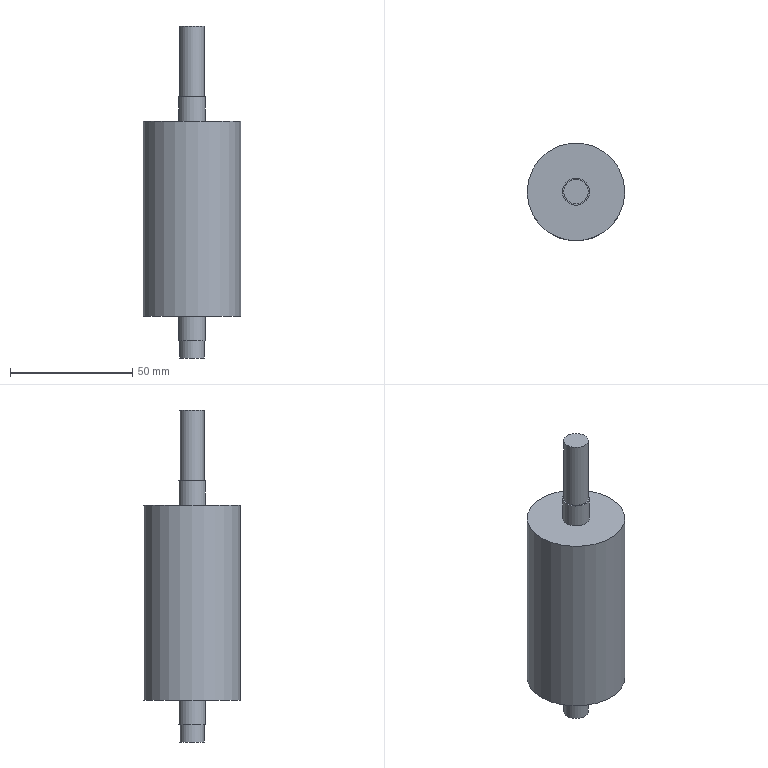Part | NX | 1 solid | 11 faces | box 40 x 40 x 136 mm | volume 105259 mm3 | plane 6 | cylinder 5 | commonest cylinder face diameters 10 x2 11 x2 40 x1
STEP:
#1=CARTESIAN_POINT('',(20.,0.,-40.));
#2=VERTEX_POINT('',#1);
#3=CARTESIAN_POINT('',(0.,0.,-40.));
#4=DIRECTION('',(0.,0.,1.));
#5=DIRECTION('',(1.,0.,0.));
#6=AXIS2_PLACEMENT_3D('',#3,#4,#5);
#7=CIRCLE('',#6,20.);
#8=EDGE_CURVE('',#2,#2,#7,.T.);
#9=ORIENTED_EDGE('',*,*,#8,.F.);
#10=EDGE_LOOP('',(#9));
#11=FACE_BOUND('',#10,.T.);
#12=CARTESIAN_POINT('',(5.5,0.,-40.));
#13=VERTEX_POINT('',#12);
#14=CARTESIAN_POINT('',(0.,0.,-40.));
#15=DIRECTION('',(0.,0.,1.));
#16=DIRECTION('',(1.,0.,0.));
#17=AXIS2_PLACEMENT_3D('',#14,#15,#16);
#18=CIRCLE('',#17,5.5);
#19=EDGE_CURVE('',#13,#13,#18,.F.);
#20=ORIENTED_EDGE('',*,*,#19,.F.);
#21=EDGE_LOOP('',(#20));
#22=FACE_BOUND('',#21,.T.);
#23=CARTESIAN_POINT('',(0.,0.,-40.));
#24=DIRECTION('',(0.,0.,1.));
#25=DIRECTION('',(1.,0.,0.));
#26=AXIS2_PLACEMENT_3D('',#23,#24,#25);
#27=PLANE('',#26);
#28=ADVANCED_FACE('',(#11,#22),#27,.F.);
#29=CARTESIAN_POINT('',(20.,0.,40.));
#30=VERTEX_POINT('',#29);
#31=CARTESIAN_POINT('',(0.,0.,40.));
#32=DIRECTION('',(0.,0.,1.));
#33=DIRECTION('',(1.,0.,0.));
#34=AXIS2_PLACEMENT_3D('',#31,#32,#33);
#35=CIRCLE('',#34,20.);
#36=EDGE_CURVE('',#30,#30,#35,.T.);
#37=ORIENTED_EDGE('',*,*,#36,.F.);
#38=EDGE_LOOP('',(#37));
#39=FACE_BOUND('',#38,.T.);
#40=ORIENTED_EDGE('',*,*,#8,.T.);
#41=EDGE_LOOP('',(#40));
#42=FACE_BOUND('',#41,.T.);
#43=CARTESIAN_POINT('',(0.,0.,40.));
#44=DIRECTION('',(0.,0.,-1.));
#45=DIRECTION('',(-1.,0.,0.));
#46=AXIS2_PLACEMENT_3D('',#43,#44,#45);
#47=CYLINDRICAL_SURFACE('',#46,20.);
#48=ADVANCED_FACE('',(#39,#42),#47,.T.);
#49=CARTESIAN_POINT('',(5.5,0.,40.));
#50=VERTEX_POINT('',#49);
#51=CARTESIAN_POINT('',(0.,0.,40.));
#52=DIRECTION('',(0.,0.,1.));
#53=DIRECTION('',(1.,0.,0.));
#54=AXIS2_PLACEMENT_3D('',#51,#52,#53);
#55=CIRCLE('',#54,5.5);
#56=EDGE_CURVE('',#50,#50,#55,.T.);
#57=ORIENTED_EDGE('',*,*,#56,.F.);
#58=EDGE_LOOP('',(#57));
#59=FACE_BOUND('',#58,.T.);
#60=ORIENTED_EDGE('',*,*,#36,.T.);
#61=EDGE_LOOP('',(#60));
#62=FACE_BOUND('',#61,.T.);
#63=CARTESIAN_POINT('',(0.,0.,40.));
#64=DIRECTION('',(0.,0.,1.));
#65=DIRECTION('',(1.,0.,0.));
#66=AXIS2_PLACEMENT_3D('',#63,#64,#65);
#67=PLANE('',#66);
#68=ADVANCED_FACE('',(#59,#62),#67,.T.);
#69=CARTESIAN_POINT('',(-5.5,0.,-50.));
#70=VERTEX_POINT('',#69);
#71=CARTESIAN_POINT('',(0.,0.,-50.));
#72=DIRECTION('',(0.,0.,-1.));
#73=DIRECTION('',(-1.,0.,0.));
#74=AXIS2_PLACEMENT_3D('',#71,#72,#73);
#75=CIRCLE('',#74,5.5);
#76=EDGE_CURVE('',#70,#70,#75,.T.);
#77=ORIENTED_EDGE('',*,*,#76,.F.);
#78=EDGE_LOOP('',(#77));
#79=FACE_BOUND('',#78,.T.);
#80=ORIENTED_EDGE('',*,*,#19,.T.);
#81=EDGE_LOOP('',(#80));
#82=FACE_BOUND('',#81,.T.);
#83=CARTESIAN_POINT('',(0.,0.,-50.));
#84=DIRECTION('',(0.,0.,1.));
#85=DIRECTION('',(1.,0.,0.));
#86=AXIS2_PLACEMENT_3D('',#83,#84,#85);
#87=CYLINDRICAL_SURFACE('',#86,5.5);
#88=ADVANCED_FACE('',(#79,#82),#87,.T.);
#89=CARTESIAN_POINT('',(-5.,0.,-50.));
#90=VERTEX_POINT('',#89);
#91=CARTESIAN_POINT('',(0.,0.,-50.));
#92=DIRECTION('',(0.,0.,-1.));
#93=DIRECTION('',(-1.,0.,0.));
#94=AXIS2_PLACEMENT_3D('',#91,#92,#93);
#95=CIRCLE('',#94,5.);
#96=EDGE_CURVE('',#90,#90,#95,.F.);
#97=ORIENTED_EDGE('',*,*,#96,.T.);
#98=EDGE_LOOP('',(#97));
#99=FACE_BOUND('',#98,.T.);
#100=ORIENTED_EDGE('',*,*,#76,.T.);
#101=EDGE_LOOP('',(#100));
#102=FACE_BOUND('',#101,.T.);
#103=CARTESIAN_POINT('',(0.,0.,-50.));
#104=DIRECTION('',(0.,0.,-1.));
#105=DIRECTION('',(-1.,0.,0.));
#106=AXIS2_PLACEMENT_3D('',#103,#104,#105);
#107=PLANE('',#106);
#108=ADVANCED_FACE('',(#99,#102),#107,.T.);
#109=CARTESIAN_POINT('',(5.,0.,-57.));
#110=VERTEX_POINT('',#109);
#111=CARTESIAN_POINT('',(0.,0.,-57.));
#112=DIRECTION('',(0.,0.,1.));
#113=DIRECTION('',(1.,0.,0.));
#114=AXIS2_PLACEMENT_3D('',#111,#112,#113);
#115=CIRCLE('',#114,5.);
#116=EDGE_CURVE('',#110,#110,#115,.T.);
#117=ORIENTED_EDGE('',*,*,#116,.F.);
#118=EDGE_LOOP('',(#117));
#119=FACE_BOUND('',#118,.T.);
#120=CARTESIAN_POINT('',(0.,0.,-57.));
#121=DIRECTION('',(0.,0.,1.));
#122=DIRECTION('',(1.,0.,0.));
#123=AXIS2_PLACEMENT_3D('',#120,#121,#122);
#124=PLANE('',#123);
#125=ADVANCED_FACE('',(#119),#124,.F.);
#126=ORIENTED_EDGE('',*,*,#96,.F.);
#127=EDGE_LOOP('',(#126));
#128=FACE_BOUND('',#127,.T.);
#129=ORIENTED_EDGE('',*,*,#116,.T.);
#130=EDGE_LOOP('',(#129));
#131=FACE_BOUND('',#130,.T.);
#132=CARTESIAN_POINT('',(0.,0.,-57.));
#133=DIRECTION('',(0.,0.,1.));
#134=DIRECTION('',(1.,0.,0.));
#135=AXIS2_PLACEMENT_3D('',#132,#133,#134);
#136=CYLINDRICAL_SURFACE('',#135,5.);
#137=ADVANCED_FACE('',(#128,#131),#136,.T.);
#138=CARTESIAN_POINT('',(-5.5,0.,50.));
#139=VERTEX_POINT('',#138);
#140=CARTESIAN_POINT('',(0.,0.,50.));
#141=DIRECTION('',(0.,0.,-1.));
#142=DIRECTION('',(-1.,0.,0.));
#143=AXIS2_PLACEMENT_3D('',#140,#141,#142);
#144=CIRCLE('',#143,5.5);
#145=EDGE_CURVE('',#139,#139,#144,.T.);
#146=ORIENTED_EDGE('',*,*,#145,.T.);
#147=EDGE_LOOP('',(#146));
#148=FACE_BOUND('',#147,.T.);
#149=ORIENTED_EDGE('',*,*,#56,.T.);
#150=EDGE_LOOP('',(#149));
#151=FACE_BOUND('',#150,.T.);
#152=CARTESIAN_POINT('',(0.,0.,50.));
#153=DIRECTION('',(0.,0.,-1.));
#154=DIRECTION('',(-1.,0.,0.));
#155=AXIS2_PLACEMENT_3D('',#152,#153,#154);
#156=CYLINDRICAL_SURFACE('',#155,5.5);
#157=ADVANCED_FACE('',(#148,#151),#156,.T.);
#158=CARTESIAN_POINT('',(5.,0.,50.));
#159=VERTEX_POINT('',#158);
#160=CARTESIAN_POINT('',(0.,0.,50.));
#161=DIRECTION('',(0.,0.,1.));
#162=DIRECTION('',(1.,0.,0.));
#163=AXIS2_PLACEMENT_3D('',#160,#161,#162);
#164=CIRCLE('',#163,5.);
#165=EDGE_CURVE('',#159,#159,#164,.F.);
#166=ORIENTED_EDGE('',*,*,#165,.T.);
#167=EDGE_LOOP('',(#166));
#168=FACE_BOUND('',#167,.T.);
#169=ORIENTED_EDGE('',*,*,#145,.F.);
#170=EDGE_LOOP('',(#169));
#171=FACE_BOUND('',#170,.T.);
#172=CARTESIAN_POINT('',(0.,0.,50.));
#173=DIRECTION('',(0.,0.,1.));
#174=DIRECTION('',(-1.,0.,0.));
#175=AXIS2_PLACEMENT_3D('',#172,#173,#174);
#176=PLANE('',#175);
#177=ADVANCED_FACE('',(#168,#171),#176,.T.);
#178=CARTESIAN_POINT('',(5.,0.,79.));
#179=VERTEX_POINT('',#178);
#180=CARTESIAN_POINT('',(0.,0.,79.));
#181=DIRECTION('',(0.,0.,1.));
#182=DIRECTION('',(1.,0.,0.));
#183=AXIS2_PLACEMENT_3D('',#180,#181,#182);
#184=CIRCLE('',#183,5.);
#185=EDGE_CURVE('',#179,#179,#184,.T.);
#186=ORIENTED_EDGE('',*,*,#185,.T.);
#187=EDGE_LOOP('',(#186));
#188=FACE_BOUND('',#187,.T.);
#189=CARTESIAN_POINT('',(0.,0.,79.));
#190=DIRECTION('',(0.,0.,1.));
#191=DIRECTION('',(1.,0.,0.));
#192=AXIS2_PLACEMENT_3D('',#189,#190,#191);
#193=PLANE('',#192);
#194=ADVANCED_FACE('',(#188),#193,.T.);
#195=ORIENTED_EDGE('',*,*,#165,.F.);
#196=EDGE_LOOP('',(#195));
#197=FACE_BOUND('',#196,.T.);
#198=ORIENTED_EDGE('',*,*,#185,.F.);
#199=EDGE_LOOP('',(#198));
#200=FACE_BOUND('',#199,.T.);
#201=CARTESIAN_POINT('',(0.,0.,-57.));
#202=DIRECTION('',(0.,0.,1.));
#203=DIRECTION('',(1.,0.,0.));
#204=AXIS2_PLACEMENT_3D('',#201,#202,#203);
#205=CYLINDRICAL_SURFACE('',#204,5.);
#206=ADVANCED_FACE('',(#197,#200),#205,.T.);
#207=CLOSED_SHELL('',(#28,#48,#68,#88,#108,#125,#137,#157,#177,#194,#206));
#208=MANIFOLD_SOLID_BREP('',#207);
#209=(LENGTH_UNIT()NAMED_UNIT(*)SI_UNIT(.MILLI.,.METRE.));
#210=UNCERTAINTY_MEASURE_WITH_UNIT(LENGTH_MEASURE(0.00001),#209,'','');
#211=(NAMED_UNIT(*)PLANE_ANGLE_UNIT()SI_UNIT($,.RADIAN.));
#212=(NAMED_UNIT(*)SI_UNIT($,.STERADIAN.)SOLID_ANGLE_UNIT());
#213=(GEOMETRIC_REPRESENTATION_CONTEXT(3)GLOBAL_UNCERTAINTY_ASSIGNED_CONTEXT((#210))GLOBAL_UNIT_ASSIGNED_CONTEXT((#209,#211,#212))REPRESENTATION_CONTEXT('',''));
#214=ADVANCED_BREP_SHAPE_REPRESENTATION('',(#208),#213);